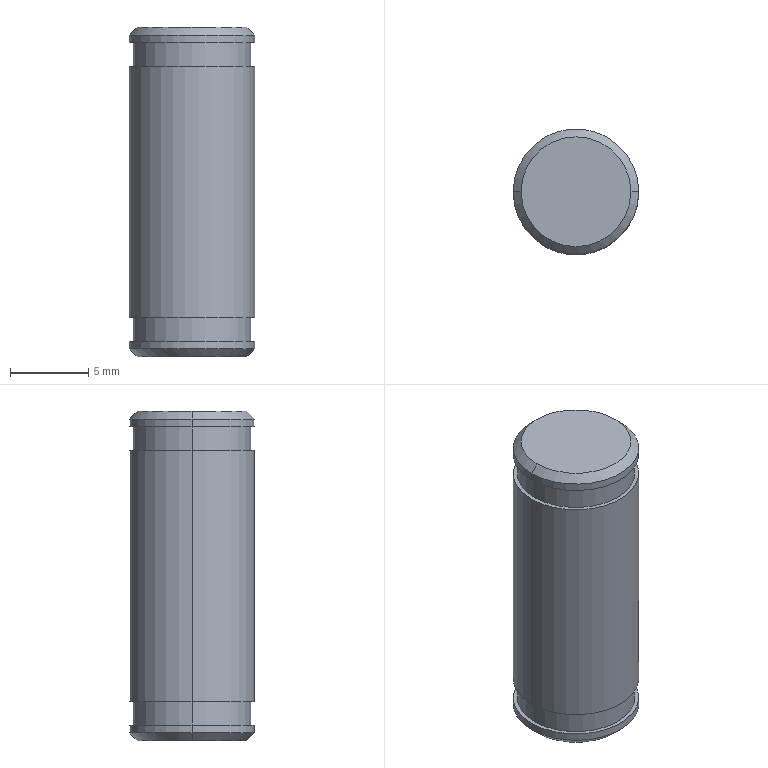Part | SolidWorks | features ICE 2, Chamfer 1, Extrusion 1, MirrorPattern 1 | 1 solid | 20 faces | box 8 x 8 x 21 mm | volume 1031 mm3 | cylinder 10 | plane 6 | cone 4 | commonest cylinder face diameters 8 x6 7.5 x4
STEP:
#1=CARTESIAN_POINT('',(-3.5,0.,-10.5));
#2=VERTEX_POINT('',#1);
#3=CARTESIAN_POINT('',(3.5,0.,-10.5));
#4=VERTEX_POINT('',#3);
#5=CARTESIAN_POINT('',(0.,0.,-10.5));
#6=DIRECTION('',(0.,0.,-1.));
#7=DIRECTION('',(-1.,0.,0.));
#8=AXIS2_PLACEMENT_3D('',#5,#6,#7);
#9=CIRCLE('',#8,3.5);
#10=EDGE_CURVE('',#2,#4,#9,.T.);
#11=ORIENTED_EDGE('',*,*,#10,.F.);
#12=CARTESIAN_POINT('',(-4.,0.,-10.));
#13=VERTEX_POINT('',#12);
#14=CARTESIAN_POINT('',(-4.,0.,-10.));
#15=DIRECTION('',(-0.7071,0.,0.7071));
#16=VECTOR('',#15,1000.);
#17=LINE('',#14,#16);
#18=EDGE_CURVE('',#2,#13,#17,.T.);
#19=ORIENTED_EDGE('',*,*,#18,.T.);
#20=CARTESIAN_POINT('',(4.,0.,-10.));
#21=VERTEX_POINT('',#20);
#22=CARTESIAN_POINT('',(0.,0.,-10.));
#23=DIRECTION('',(0.,0.,1.));
#24=DIRECTION('',(-1.,0.,0.));
#25=AXIS2_PLACEMENT_3D('',#22,#23,#24);
#26=CIRCLE('',#25,4.);
#27=EDGE_CURVE('',#21,#13,#26,.T.);
#28=ORIENTED_EDGE('',*,*,#27,.F.);
#29=CARTESIAN_POINT('',(4.,0.,-10.));
#30=DIRECTION('',(0.7071,0.,0.7071));
#31=VECTOR('',#30,1000.);
#32=LINE('',#29,#31);
#33=EDGE_CURVE('',#4,#21,#32,.T.);
#34=ORIENTED_EDGE('',*,*,#33,.F.);
#35=EDGE_LOOP('',(#11,#19,#28,#34));
#36=FACE_OUTER_BOUND('',#35,.T.);
#37=CARTESIAN_POINT('',(0.,0.,-10.));
#38=DIRECTION('',(0.,0.,1.));
#39=DIRECTION('',(1.,0.,0.));
#40=AXIS2_PLACEMENT_3D('',#37,#38,#39);
#41=CONICAL_SURFACE('',#40,4.,0.7854);
#42=ADVANCED_FACE('',(#36),#41,.T.);
#43=ORIENTED_EDGE('',*,*,#27,.T.);
#44=CARTESIAN_POINT('',(-4.,0.,-9.5));
#45=VERTEX_POINT('',#44);
#46=CARTESIAN_POINT('',(-4.,0.,-10.5));
#47=DIRECTION('',(0.,0.,1.));
#48=VECTOR('',#47,1000.);
#49=LINE('',#46,#48);
#50=EDGE_CURVE('',#13,#45,#49,.T.);
#51=ORIENTED_EDGE('',*,*,#50,.T.);
#52=CARTESIAN_POINT('',(4.,0.,-9.5));
#53=VERTEX_POINT('',#52);
#54=CARTESIAN_POINT('',(0.,0.,-9.5));
#55=DIRECTION('',(0.,0.,1.));
#56=DIRECTION('',(1.,0.,0.));
#57=AXIS2_PLACEMENT_3D('',#54,#55,#56);
#58=CIRCLE('',#57,4.);
#59=EDGE_CURVE('',#53,#45,#58,.T.);
#60=ORIENTED_EDGE('',*,*,#59,.F.);
#61=CARTESIAN_POINT('',(4.,0.,-10.5));
#62=DIRECTION('',(0.,0.,1.));
#63=VECTOR('',#62,1000.);
#64=LINE('',#61,#63);
#65=EDGE_CURVE('',#21,#53,#64,.T.);
#66=ORIENTED_EDGE('',*,*,#65,.F.);
#67=EDGE_LOOP('',(#43,#51,#60,#66));
#68=FACE_OUTER_BOUND('',#67,.T.);
#69=CARTESIAN_POINT('',(0.,0.,-10.5));
#70=DIRECTION('',(0.,0.,1.));
#71=DIRECTION('',(1.,0.,0.));
#72=AXIS2_PLACEMENT_3D('',#69,#70,#71);
#73=CYLINDRICAL_SURFACE('',#72,4.);
#74=ADVANCED_FACE('',(#68),#73,.T.);
#75=CARTESIAN_POINT('',(3.75,0.,-9.5));
#76=VERTEX_POINT('',#75);
#77=CARTESIAN_POINT('',(-3.75,0.,-9.5));
#78=VERTEX_POINT('',#77);
#79=CARTESIAN_POINT('',(0.,0.,-9.5));
#80=DIRECTION('',(0.,0.,1.));
#81=DIRECTION('',(1.,0.,0.));
#82=AXIS2_PLACEMENT_3D('',#79,#80,#81);
#83=CIRCLE('',#82,3.75);
#84=EDGE_CURVE('',#76,#78,#83,.T.);
#85=ORIENTED_EDGE('',*,*,#84,.T.);
#86=CARTESIAN_POINT('',(-3.75,0.,-8.));
#87=VERTEX_POINT('',#86);
#88=CARTESIAN_POINT('',(-3.75,0.,-9.5));
#89=DIRECTION('',(0.,0.,1.));
#90=VECTOR('',#89,1000.);
#91=LINE('',#88,#90);
#92=EDGE_CURVE('',#78,#87,#91,.T.);
#93=ORIENTED_EDGE('',*,*,#92,.T.);
#94=CARTESIAN_POINT('',(3.75,0.,-8.));
#95=VERTEX_POINT('',#94);
#96=CARTESIAN_POINT('',(0.,0.,-8.));
#97=DIRECTION('',(0.,0.,1.));
#98=DIRECTION('',(1.,0.,0.));
#99=AXIS2_PLACEMENT_3D('',#96,#97,#98);
#100=CIRCLE('',#99,3.75);
#101=EDGE_CURVE('',#95,#87,#100,.T.);
#102=ORIENTED_EDGE('',*,*,#101,.F.);
#103=CARTESIAN_POINT('',(3.75,0.,-9.5));
#104=DIRECTION('',(0.,0.,1.));
#105=VECTOR('',#104,1000.);
#106=LINE('',#103,#105);
#107=EDGE_CURVE('',#76,#95,#106,.T.);
#108=ORIENTED_EDGE('',*,*,#107,.F.);
#109=EDGE_LOOP('',(#85,#93,#102,#108));
#110=FACE_OUTER_BOUND('',#109,.T.);
#111=CARTESIAN_POINT('',(0.,0.,-9.5));
#112=DIRECTION('',(0.,0.,1.));
#113=DIRECTION('',(1.,0.,0.));
#114=AXIS2_PLACEMENT_3D('',#111,#112,#113);
#115=CYLINDRICAL_SURFACE('',#114,3.75);
#116=ADVANCED_FACE('',(#110),#115,.T.);
#117=CARTESIAN_POINT('',(3.5,0.,10.5));
#118=VERTEX_POINT('',#117);
#119=CARTESIAN_POINT('',(-3.5,0.,10.5));
#120=VERTEX_POINT('',#119);
#121=CARTESIAN_POINT('',(0.,0.,10.5));
#122=DIRECTION('',(0.,0.,1.));
#123=DIRECTION('',(1.,0.,0.));
#124=AXIS2_PLACEMENT_3D('',#121,#122,#123);
#125=CIRCLE('',#124,3.5);
#126=EDGE_CURVE('',#118,#120,#125,.T.);
#127=ORIENTED_EDGE('',*,*,#126,.F.);
#128=CARTESIAN_POINT('',(4.,0.,10.));
#129=VERTEX_POINT('',#128);
#130=CARTESIAN_POINT('',(3.5,0.,10.5));
#131=DIRECTION('',(0.7071,0.,-0.7071));
#132=VECTOR('',#131,1000.);
#133=LINE('',#130,#132);
#134=EDGE_CURVE('',#118,#129,#133,.T.);
#135=ORIENTED_EDGE('',*,*,#134,.T.);
#136=CARTESIAN_POINT('',(-4.,0.,10.));
#137=VERTEX_POINT('',#136);
#138=CARTESIAN_POINT('',(0.,0.,10.));
#139=DIRECTION('',(0.,0.,-1.));
#140=DIRECTION('',(1.,0.,0.));
#141=AXIS2_PLACEMENT_3D('',#138,#139,#140);
#142=CIRCLE('',#141,4.);
#143=EDGE_CURVE('',#137,#129,#142,.T.);
#144=ORIENTED_EDGE('',*,*,#143,.F.);
#145=CARTESIAN_POINT('',(-3.5,0.,10.5));
#146=DIRECTION('',(-0.7071,0.,-0.7071));
#147=VECTOR('',#146,1000.);
#148=LINE('',#145,#147);
#149=EDGE_CURVE('',#120,#137,#148,.T.);
#150=ORIENTED_EDGE('',*,*,#149,.F.);
#151=EDGE_LOOP('',(#127,#135,#144,#150));
#152=FACE_OUTER_BOUND('',#151,.T.);
#153=CARTESIAN_POINT('',(0.,0.,10.5));
#154=DIRECTION('',(0.,0.,-1.));
#155=DIRECTION('',(-1.,0.,0.));
#156=AXIS2_PLACEMENT_3D('',#153,#154,#155);
#157=CONICAL_SURFACE('',#156,3.5,0.7854);
#158=ADVANCED_FACE('',(#152),#157,.T.);
#159=ORIENTED_EDGE('',*,*,#143,.T.);
#160=CARTESIAN_POINT('',(4.,0.,9.5));
#161=VERTEX_POINT('',#160);
#162=CARTESIAN_POINT('',(4.,0.,10.5));
#163=DIRECTION('',(0.,0.,-1.));
#164=VECTOR('',#163,1000.);
#165=LINE('',#162,#164);
#166=EDGE_CURVE('',#129,#161,#165,.T.);
#167=ORIENTED_EDGE('',*,*,#166,.T.);
#168=CARTESIAN_POINT('',(-4.,0.,9.5));
#169=VERTEX_POINT('',#168);
#170=CARTESIAN_POINT('',(0.,0.,9.5));
#171=DIRECTION('',(0.,0.,1.));
#172=DIRECTION('',(1.,0.,0.));
#173=AXIS2_PLACEMENT_3D('',#170,#171,#172);
#174=CIRCLE('',#173,4.);
#175=EDGE_CURVE('',#161,#169,#174,.T.);
#176=ORIENTED_EDGE('',*,*,#175,.T.);
#177=CARTESIAN_POINT('',(-4.,0.,10.5));
#178=DIRECTION('',(0.,0.,-1.));
#179=VECTOR('',#178,1000.);
#180=LINE('',#177,#179);
#181=EDGE_CURVE('',#137,#169,#180,.T.);
#182=ORIENTED_EDGE('',*,*,#181,.F.);
#183=EDGE_LOOP('',(#159,#167,#176,#182));
#184=FACE_OUTER_BOUND('',#183,.T.);
#185=CARTESIAN_POINT('',(0.,0.,10.5));
#186=DIRECTION('',(0.,0.,-1.));
#187=DIRECTION('',(-1.,0.,0.));
#188=AXIS2_PLACEMENT_3D('',#185,#186,#187);
#189=CYLINDRICAL_SURFACE('',#188,4.);
#190=ADVANCED_FACE('',(#184),#189,.T.);
#191=CARTESIAN_POINT('',(3.75,0.,9.5));
#192=VERTEX_POINT('',#191);
#193=CARTESIAN_POINT('',(-3.75,0.,9.5));
#194=VERTEX_POINT('',#193);
#195=CARTESIAN_POINT('',(0.,0.,9.5));
#196=DIRECTION('',(0.,0.,1.));
#197=DIRECTION('',(1.,0.,0.));
#198=AXIS2_PLACEMENT_3D('',#195,#196,#197);
#199=CIRCLE('',#198,3.75);
#200=EDGE_CURVE('',#192,#194,#199,.T.);
#201=ORIENTED_EDGE('',*,*,#200,.F.);
#202=CARTESIAN_POINT('',(3.75,0.,8.));
#203=VERTEX_POINT('',#202);
#204=CARTESIAN_POINT('',(3.75,0.,9.5));
#205=DIRECTION('',(0.,0.,-1.));
#206=VECTOR('',#205,1000.);
#207=LINE('',#204,#206);
#208=EDGE_CURVE('',#192,#203,#207,.T.);
#209=ORIENTED_EDGE('',*,*,#208,.T.);
#210=CARTESIAN_POINT('',(-3.75,0.,8.));
#211=VERTEX_POINT('',#210);
#212=CARTESIAN_POINT('',(0.,0.,8.));
#213=DIRECTION('',(0.,0.,1.));
#214=DIRECTION('',(1.,0.,0.));
#215=AXIS2_PLACEMENT_3D('',#212,#213,#214);
#216=CIRCLE('',#215,3.75);
#217=EDGE_CURVE('',#203,#211,#216,.T.);
#218=ORIENTED_EDGE('',*,*,#217,.T.);
#219=CARTESIAN_POINT('',(-3.75,0.,9.5));
#220=DIRECTION('',(0.,0.,-1.));
#221=VECTOR('',#220,1000.);
#222=LINE('',#219,#221);
#223=EDGE_CURVE('',#194,#211,#222,.T.);
#224=ORIENTED_EDGE('',*,*,#223,.F.);
#225=EDGE_LOOP('',(#201,#209,#218,#224));
#226=FACE_OUTER_BOUND('',#225,.T.);
#227=CARTESIAN_POINT('',(0.,0.,9.5));
#228=DIRECTION('',(0.,0.,-1.));
#229=DIRECTION('',(-1.,0.,0.));
#230=AXIS2_PLACEMENT_3D('',#227,#228,#229);
#231=CYLINDRICAL_SURFACE('',#230,3.75);
#232=ADVANCED_FACE('',(#226),#231,.T.);
#233=CARTESIAN_POINT('',(4.,0.,8.));
#234=VERTEX_POINT('',#233);
#235=CARTESIAN_POINT('',(-4.,0.,8.));
#236=VERTEX_POINT('',#235);
#237=CARTESIAN_POINT('',(0.,0.,8.));
#238=DIRECTION('',(0.,0.,1.));
#239=DIRECTION('',(1.,0.,0.));
#240=AXIS2_PLACEMENT_3D('',#237,#238,#239);
#241=CIRCLE('',#240,4.);
#242=EDGE_CURVE('',#234,#236,#241,.T.);
#243=ORIENTED_EDGE('',*,*,#242,.F.);
#244=CARTESIAN_POINT('',(4.,0.,-8.));
#245=VERTEX_POINT('',#244);
#246=CARTESIAN_POINT('',(4.,0.,8.));
#247=DIRECTION('',(0.,0.,-1.));
#248=VECTOR('',#247,1000.);
#249=LINE('',#246,#248);
#250=EDGE_CURVE('',#234,#245,#249,.T.);
#251=ORIENTED_EDGE('',*,*,#250,.T.);
#252=CARTESIAN_POINT('',(-4.,0.,-8.));
#253=VERTEX_POINT('',#252);
#254=CARTESIAN_POINT('',(0.,0.,-8.));
#255=DIRECTION('',(0.,0.,1.));
#256=DIRECTION('',(1.,0.,0.));
#257=AXIS2_PLACEMENT_3D('',#254,#255,#256);
#258=CIRCLE('',#257,4.);
#259=EDGE_CURVE('',#245,#253,#258,.T.);
#260=ORIENTED_EDGE('',*,*,#259,.T.);
#261=CARTESIAN_POINT('',(-4.,0.,8.));
#262=DIRECTION('',(0.,0.,-1.));
#263=VECTOR('',#262,1000.);
#264=LINE('',#261,#263);
#265=EDGE_CURVE('',#236,#253,#264,.T.);
#266=ORIENTED_EDGE('',*,*,#265,.F.);
#267=EDGE_LOOP('',(#243,#251,#260,#266));
#268=FACE_OUTER_BOUND('',#267,.T.);
#269=CARTESIAN_POINT('',(0.,0.,8.));
#270=DIRECTION('',(0.,0.,-1.));
#271=DIRECTION('',(-1.,0.,0.));
#272=AXIS2_PLACEMENT_3D('',#269,#270,#271);
#273=CYLINDRICAL_SURFACE('',#272,4.);
#274=ADVANCED_FACE('',(#268),#273,.T.);
#275=ORIENTED_EDGE('',*,*,#250,.F.);
#276=CARTESIAN_POINT('',(0.,0.,8.));
#277=DIRECTION('',(0.,0.,1.));
#278=DIRECTION('',(1.,0.,0.));
#279=AXIS2_PLACEMENT_3D('',#276,#277,#278);
#280=CIRCLE('',#279,4.);
#281=EDGE_CURVE('',#236,#234,#280,.T.);
#282=ORIENTED_EDGE('',*,*,#281,.F.);
#283=ORIENTED_EDGE('',*,*,#265,.T.);
#284=CARTESIAN_POINT('',(0.,0.,-8.));
#285=DIRECTION('',(0.,0.,1.));
#286=DIRECTION('',(1.,0.,0.));
#287=AXIS2_PLACEMENT_3D('',#284,#285,#286);
#288=CIRCLE('',#287,4.);
#289=EDGE_CURVE('',#253,#245,#288,.T.);
#290=ORIENTED_EDGE('',*,*,#289,.T.);
#291=EDGE_LOOP('',(#275,#282,#283,#290));
#292=FACE_OUTER_BOUND('',#291,.T.);
#293=CARTESIAN_POINT('',(0.,0.,8.));
#294=DIRECTION('',(0.,0.,-1.));
#295=DIRECTION('',(-1.,0.,0.));
#296=AXIS2_PLACEMENT_3D('',#293,#294,#295);
#297=CYLINDRICAL_SURFACE('',#296,4.);
#298=ADVANCED_FACE('',(#292),#297,.T.);
#299=CARTESIAN_POINT('',(0.,0.,8.));
#300=DIRECTION('',(0.,0.,1.));
#301=DIRECTION('',(1.,0.,0.));
#302=AXIS2_PLACEMENT_3D('',#299,#300,#301);
#303=CIRCLE('',#302,3.75);
#304=EDGE_CURVE('',#211,#203,#303,.T.);
#305=ORIENTED_EDGE('',*,*,#304,.F.);
#306=ORIENTED_EDGE('',*,*,#217,.F.);
#307=EDGE_LOOP('',(#305,#306));
#308=FACE_BOUND('',#307,.T.);
#309=ORIENTED_EDGE('',*,*,#281,.T.);
#310=ORIENTED_EDGE('',*,*,#242,.T.);
#311=EDGE_LOOP('',(#309,#310));
#312=FACE_OUTER_BOUND('',#311,.T.);
#313=CARTESIAN_POINT('',(0.,0.,8.));
#314=DIRECTION('',(0.,0.,1.));
#315=DIRECTION('',(1.,0.,0.));
#316=AXIS2_PLACEMENT_3D('',#313,#314,#315);
#317=PLANE('',#316);
#318=ADVANCED_FACE('',(#308,#312),#317,.T.);
#319=ORIENTED_EDGE('',*,*,#101,.T.);
#320=CARTESIAN_POINT('',(0.,0.,-8.));
#321=DIRECTION('',(0.,0.,1.));
#322=DIRECTION('',(1.,0.,0.));
#323=AXIS2_PLACEMENT_3D('',#320,#321,#322);
#324=CIRCLE('',#323,3.75);
#325=EDGE_CURVE('',#87,#95,#324,.T.);
#326=ORIENTED_EDGE('',*,*,#325,.T.);
#327=EDGE_LOOP('',(#319,#326));
#328=FACE_BOUND('',#327,.T.);
#329=ORIENTED_EDGE('',*,*,#289,.F.);
#330=ORIENTED_EDGE('',*,*,#259,.F.);
#331=EDGE_LOOP('',(#329,#330));
#332=FACE_OUTER_BOUND('',#331,.T.);
#333=CARTESIAN_POINT('',(0.,0.,-8.));
#334=DIRECTION('',(0.,0.,1.));
#335=DIRECTION('',(1.,0.,0.));
#336=AXIS2_PLACEMENT_3D('',#333,#334,#335);
#337=PLANE('',#336);
#338=ADVANCED_FACE('',(#328,#332),#337,.F.);
#339=ORIENTED_EDGE('',*,*,#208,.F.);
#340=CARTESIAN_POINT('',(0.,0.,9.5));
#341=DIRECTION('',(0.,0.,1.));
#342=DIRECTION('',(1.,0.,0.));
#343=AXIS2_PLACEMENT_3D('',#340,#341,#342);
#344=CIRCLE('',#343,3.75);
#345=EDGE_CURVE('',#194,#192,#344,.T.);
#346=ORIENTED_EDGE('',*,*,#345,.F.);
#347=ORIENTED_EDGE('',*,*,#223,.T.);
#348=ORIENTED_EDGE('',*,*,#304,.T.);
#349=EDGE_LOOP('',(#339,#346,#347,#348));
#350=FACE_OUTER_BOUND('',#349,.T.);
#351=CARTESIAN_POINT('',(0.,0.,9.5));
#352=DIRECTION('',(0.,0.,-1.));
#353=DIRECTION('',(-1.,0.,0.));
#354=AXIS2_PLACEMENT_3D('',#351,#352,#353);
#355=CYLINDRICAL_SURFACE('',#354,3.75);
#356=ADVANCED_FACE('',(#350),#355,.T.);
#357=ORIENTED_EDGE('',*,*,#166,.F.);
#358=CARTESIAN_POINT('',(0.,0.,10.));
#359=DIRECTION('',(0.,0.,-1.));
#360=DIRECTION('',(1.,0.,0.));
#361=AXIS2_PLACEMENT_3D('',#358,#359,#360);
#362=CIRCLE('',#361,4.);
#363=EDGE_CURVE('',#129,#137,#362,.T.);
#364=ORIENTED_EDGE('',*,*,#363,.T.);
#365=ORIENTED_EDGE('',*,*,#181,.T.);
#366=CARTESIAN_POINT('',(0.,0.,9.5));
#367=DIRECTION('',(0.,0.,1.));
#368=DIRECTION('',(1.,0.,0.));
#369=AXIS2_PLACEMENT_3D('',#366,#367,#368);
#370=CIRCLE('',#369,4.);
#371=EDGE_CURVE('',#169,#161,#370,.T.);
#372=ORIENTED_EDGE('',*,*,#371,.T.);
#373=EDGE_LOOP('',(#357,#364,#365,#372));
#374=FACE_OUTER_BOUND('',#373,.T.);
#375=CARTESIAN_POINT('',(0.,0.,10.5));
#376=DIRECTION('',(0.,0.,-1.));
#377=DIRECTION('',(-1.,0.,0.));
#378=AXIS2_PLACEMENT_3D('',#375,#376,#377);
#379=CYLINDRICAL_SURFACE('',#378,4.);
#380=ADVANCED_FACE('',(#374),#379,.T.);
#381=CARTESIAN_POINT('',(0.,0.,10.5));
#382=DIRECTION('',(0.,0.,1.));
#383=DIRECTION('',(1.,0.,0.));
#384=AXIS2_PLACEMENT_3D('',#381,#382,#383);
#385=CIRCLE('',#384,3.5);
#386=EDGE_CURVE('',#120,#118,#385,.T.);
#387=ORIENTED_EDGE('',*,*,#386,.T.);
#388=ORIENTED_EDGE('',*,*,#126,.T.);
#389=EDGE_LOOP('',(#387,#388));
#390=FACE_OUTER_BOUND('',#389,.T.);
#391=CARTESIAN_POINT('',(0.,0.,10.5));
#392=DIRECTION('',(0.,0.,1.));
#393=DIRECTION('',(1.,0.,0.));
#394=AXIS2_PLACEMENT_3D('',#391,#392,#393);
#395=PLANE('',#394);
#396=ADVANCED_FACE('',(#390),#395,.T.);
#397=ORIENTED_EDGE('',*,*,#345,.T.);
#398=ORIENTED_EDGE('',*,*,#200,.T.);
#399=EDGE_LOOP('',(#397,#398));
#400=FACE_BOUND('',#399,.T.);
#401=ORIENTED_EDGE('',*,*,#371,.F.);
#402=ORIENTED_EDGE('',*,*,#175,.F.);
#403=EDGE_LOOP('',(#401,#402));
#404=FACE_OUTER_BOUND('',#403,.T.);
#405=CARTESIAN_POINT('',(0.,0.,9.5));
#406=DIRECTION('',(0.,0.,1.));
#407=DIRECTION('',(1.,0.,0.));
#408=AXIS2_PLACEMENT_3D('',#405,#406,#407);
#409=PLANE('',#408);
#410=ADVANCED_FACE('',(#400,#404),#409,.F.);
#411=ORIENTED_EDGE('',*,*,#134,.F.);
#412=ORIENTED_EDGE('',*,*,#386,.F.);
#413=ORIENTED_EDGE('',*,*,#149,.T.);
#414=ORIENTED_EDGE('',*,*,#363,.F.);
#415=EDGE_LOOP('',(#411,#412,#413,#414));
#416=FACE_OUTER_BOUND('',#415,.T.);
#417=CARTESIAN_POINT('',(0.,0.,10.5));
#418=DIRECTION('',(0.,0.,-1.));
#419=DIRECTION('',(-1.,0.,0.));
#420=AXIS2_PLACEMENT_3D('',#417,#418,#419);
#421=CONICAL_SURFACE('',#420,3.5,0.7854);
#422=ADVANCED_FACE('',(#416),#421,.T.);
#423=ORIENTED_EDGE('',*,*,#92,.F.);
#424=CARTESIAN_POINT('',(0.,0.,-9.5));
#425=DIRECTION('',(0.,0.,1.));
#426=DIRECTION('',(1.,0.,0.));
#427=AXIS2_PLACEMENT_3D('',#424,#425,#426);
#428=CIRCLE('',#427,3.75);
#429=EDGE_CURVE('',#78,#76,#428,.T.);
#430=ORIENTED_EDGE('',*,*,#429,.T.);
#431=ORIENTED_EDGE('',*,*,#107,.T.);
#432=ORIENTED_EDGE('',*,*,#325,.F.);
#433=EDGE_LOOP('',(#423,#430,#431,#432));
#434=FACE_OUTER_BOUND('',#433,.T.);
#435=CARTESIAN_POINT('',(0.,0.,-9.5));
#436=DIRECTION('',(0.,0.,1.));
#437=DIRECTION('',(1.,0.,0.));
#438=AXIS2_PLACEMENT_3D('',#435,#436,#437);
#439=CYLINDRICAL_SURFACE('',#438,3.75);
#440=ADVANCED_FACE('',(#434),#439,.T.);
#441=ORIENTED_EDGE('',*,*,#50,.F.);
#442=CARTESIAN_POINT('',(0.,0.,-10.));
#443=DIRECTION('',(0.,0.,1.));
#444=DIRECTION('',(-1.,0.,0.));
#445=AXIS2_PLACEMENT_3D('',#442,#443,#444);
#446=CIRCLE('',#445,4.);
#447=EDGE_CURVE('',#13,#21,#446,.T.);
#448=ORIENTED_EDGE('',*,*,#447,.T.);
#449=ORIENTED_EDGE('',*,*,#65,.T.);
#450=CARTESIAN_POINT('',(0.,0.,-9.5));
#451=DIRECTION('',(0.,0.,1.));
#452=DIRECTION('',(1.,0.,0.));
#453=AXIS2_PLACEMENT_3D('',#450,#451,#452);
#454=CIRCLE('',#453,4.);
#455=EDGE_CURVE('',#45,#53,#454,.T.);
#456=ORIENTED_EDGE('',*,*,#455,.F.);
#457=EDGE_LOOP('',(#441,#448,#449,#456));
#458=FACE_OUTER_BOUND('',#457,.T.);
#459=CARTESIAN_POINT('',(0.,0.,-10.5));
#460=DIRECTION('',(0.,0.,1.));
#461=DIRECTION('',(1.,0.,0.));
#462=AXIS2_PLACEMENT_3D('',#459,#460,#461);
#463=CYLINDRICAL_SURFACE('',#462,4.);
#464=ADVANCED_FACE('',(#458),#463,.T.);
#465=CARTESIAN_POINT('',(0.,0.,-10.5));
#466=DIRECTION('',(0.,0.,-1.));
#467=DIRECTION('',(-1.,0.,0.));
#468=AXIS2_PLACEMENT_3D('',#465,#466,#467);
#469=CIRCLE('',#468,3.5);
#470=EDGE_CURVE('',#4,#2,#469,.T.);
#471=ORIENTED_EDGE('',*,*,#470,.T.);
#472=ORIENTED_EDGE('',*,*,#10,.T.);
#473=EDGE_LOOP('',(#471,#472));
#474=FACE_OUTER_BOUND('',#473,.T.);
#475=CARTESIAN_POINT('',(0.,0.,-10.5));
#476=DIRECTION('',(0.,0.,-1.));
#477=DIRECTION('',(1.,0.,0.));
#478=AXIS2_PLACEMENT_3D('',#475,#476,#477);
#479=PLANE('',#478);
#480=ADVANCED_FACE('',(#474),#479,.T.);
#481=ORIENTED_EDGE('',*,*,#84,.F.);
#482=ORIENTED_EDGE('',*,*,#429,.F.);
#483=EDGE_LOOP('',(#481,#482));
#484=FACE_BOUND('',#483,.T.);
#485=ORIENTED_EDGE('',*,*,#59,.T.);
#486=ORIENTED_EDGE('',*,*,#455,.T.);
#487=EDGE_LOOP('',(#485,#486));
#488=FACE_OUTER_BOUND('',#487,.T.);
#489=CARTESIAN_POINT('',(0.,0.,-9.5));
#490=DIRECTION('',(0.,0.,-1.));
#491=DIRECTION('',(1.,0.,0.));
#492=AXIS2_PLACEMENT_3D('',#489,#490,#491);
#493=PLANE('',#492);
#494=ADVANCED_FACE('',(#484,#488),#493,.F.);
#495=ORIENTED_EDGE('',*,*,#18,.F.);
#496=ORIENTED_EDGE('',*,*,#470,.F.);
#497=ORIENTED_EDGE('',*,*,#33,.T.);
#498=ORIENTED_EDGE('',*,*,#447,.F.);
#499=EDGE_LOOP('',(#495,#496,#497,#498));
#500=FACE_OUTER_BOUND('',#499,.T.);
#501=CARTESIAN_POINT('',(0.,0.,-10.));
#502=DIRECTION('',(0.,0.,1.));
#503=DIRECTION('',(1.,0.,0.));
#504=AXIS2_PLACEMENT_3D('',#501,#502,#503);
#505=CONICAL_SURFACE('',#504,4.,0.7854);
#506=ADVANCED_FACE('',(#500),#505,.T.);
#507=CLOSED_SHELL('',(#42,#74,#116,#158,#190,#232,#274,#298,#318,#338,#356,#380,#396,#410,#422,#440,#464,#480,#494,#506));
#508=MANIFOLD_SOLID_BREP('',#507);
#509=CARTESIAN_POINT('',(0.,0.,0.));
#510=DIRECTION('',(0.,0.,1.));
#511=DIRECTION('',(1.,0.,0.));
#512=AXIS2_PLACEMENT_3D('',#509,#510,#511);
#513=(LENGTH_UNIT()NAMED_UNIT(*)SI_UNIT(.MILLI.,.METRE.));
#514=UNCERTAINTY_MEASURE_WITH_UNIT(LENGTH_MEASURE(0.00001),#513,'','');
#515=(NAMED_UNIT(*)PLANE_ANGLE_UNIT()SI_UNIT($,.RADIAN.));
#516=(NAMED_UNIT(*)SI_UNIT($,.STERADIAN.)SOLID_ANGLE_UNIT());
#517=(GEOMETRIC_REPRESENTATION_CONTEXT(3)GLOBAL_UNCERTAINTY_ASSIGNED_CONTEXT((#514))GLOBAL_UNIT_ASSIGNED_CONTEXT((#513,#515,#516))REPRESENTATION_CONTEXT('',''));
#518=ADVANCED_BREP_SHAPE_REPRESENTATION('',(#508,#512),#517);